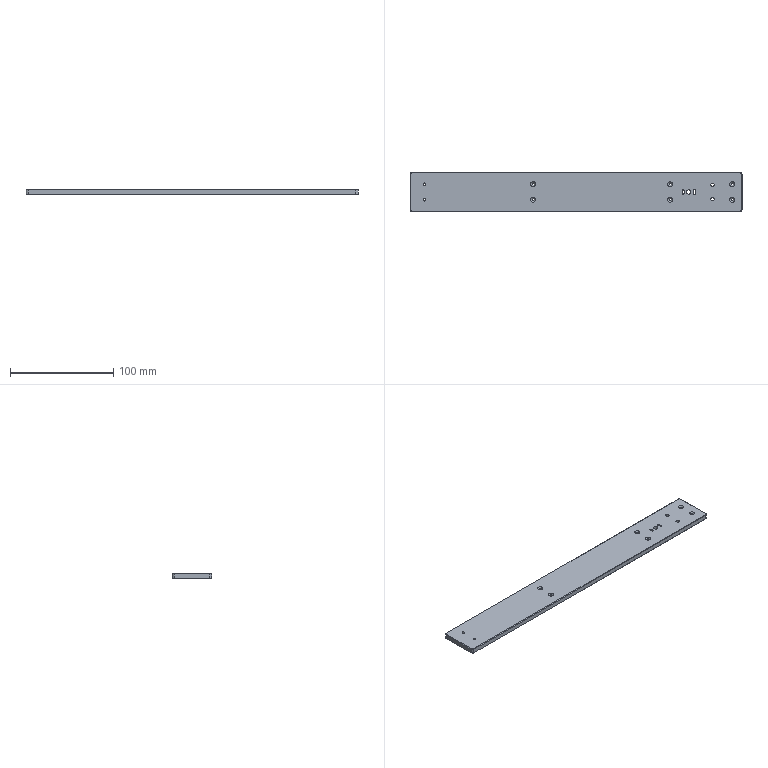CAM job | NX | 3-axis milling | part box 321 x 38 x 5 mm | stock box 327 x 44 x 5 mm
Tools:
number,name,description,diameter,corner_radius,flute_length,length,flutes
2,D10,Milling Tool-5 Parameters,10.0,0.0,50.0,75.0,2
6,D4,Milling Tool-5 Parameters,4.0,0.0,50.0,75.0,2
9,D6A45,Milling Tool-5 Parameters,6.0,0.0,3.0,3.0,2
8,D2,Milling Tool-5 Parameters,2.0,0.0,50.0,75.0,2
18,D1,Milling Tool-5 Parameters,1.0,0.0,50.0,75.0,2
Operations:
program,operation,operation_type,tool,method,geometry_group,spindle_rpm,surface_speed,feed_per_tooth,feed_cut,feed_plunge,cut_length_mm,path_length_mm,cut_time_min,machine_time_min
325-43-5毛胚-吸盘,ZLEVEL_PROFILE,ZLevelMilling,D10,METHOD,A,6500.0,326.0,0.1538,2000.0,1000.0,3835.06,3896.76,1.941,1.947
325-43-5毛胚-吸盘,ZLEVEL_PROFILE_COPY_COPY_1_COPY_COPY_1_COPY,ZLevelMilling,D2,METHOD,A,7000.0,43.0,0.0714,1000.0,1000.0,3403.68,4455.134,3.404,3.509
325-43-5毛胚-吸盘,ZLEVEL_PROFILE_COPY_COPY_1_COPY_COPY_1_COPY_COPY,ZLevelMilling,D1,METHOD,A,7000.0,43.0,0.0714,1000.0,1000.0,1617.135,1751.845,1.617,1.631
325-43-5毛胚-吸盘,ZLEVEL_PROFILE_COPY_1_COPY_COPY_COPY_COPY_COPY_COPY,ZLevelMilling,D6A45,METHOD,A,7000.0,131.0,0.0714,1000.0,1000.0,757.503,1898.703,0.7575,0.8716
325-43-5毛胚-吸盘,ZLEVEL_PROFILE_COPY_COPY_1_COPY,ZLevelMilling,D4,METHOD,A,6000.0,75.0,0.0833,1000.0,1000.0,732.581,799.281,0.7326,0.7393